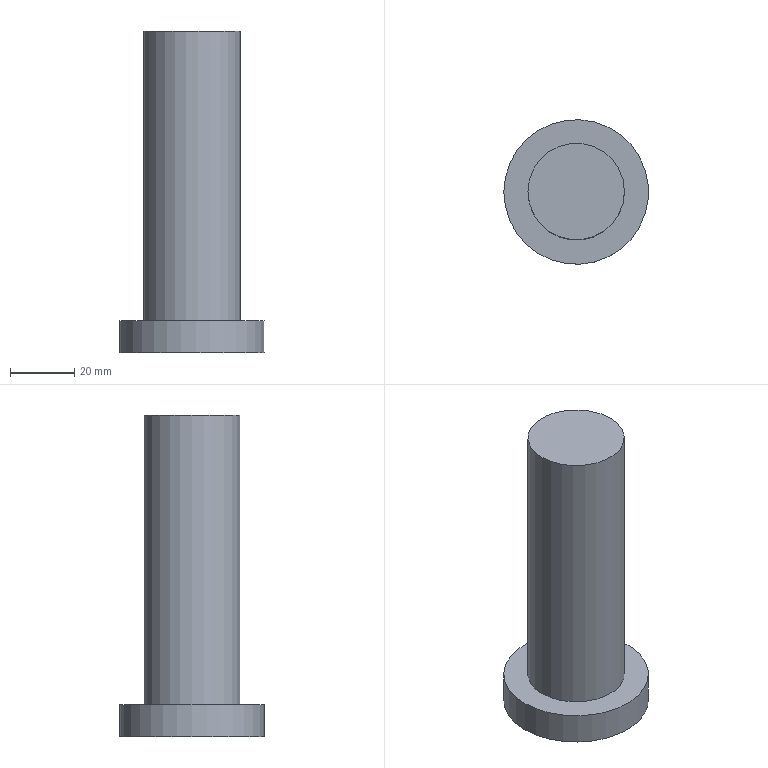Part | NX | features 侧推千斤顶缸销 2 | 1 solid | 5 faces | box 45 x 45 x 100 mm | volume 79522 mm3 | plane 3 | cylinder 2 | commonest cylinder face diameters 30 x1 45 x1
STEP:
#1=CARTESIAN_POINT('',(15.,0.,90.));
#2=VERTEX_POINT('',#1);
#3=CARTESIAN_POINT('',(0.,0.,90.));
#4=DIRECTION('',(0.,0.,1.));
#5=DIRECTION('',(1.,0.,0.));
#6=AXIS2_PLACEMENT_3D('',#3,#4,#5);
#7=CIRCLE('',#6,15.);
#8=EDGE_CURVE('',#2,#2,#7,.T.);
#9=ORIENTED_EDGE('',*,*,#8,.F.);
#10=EDGE_LOOP('',(#9));
#11=FACE_BOUND('',#10,.T.);
#12=CARTESIAN_POINT('',(-15.,0.,0.));
#13=VERTEX_POINT('',#12);
#14=CARTESIAN_POINT('',(0.,0.,0.));
#15=DIRECTION('',(0.,0.,-1.));
#16=DIRECTION('',(-1.,0.,0.));
#17=AXIS2_PLACEMENT_3D('',#14,#15,#16);
#18=CIRCLE('',#17,15.);
#19=EDGE_CURVE('',#13,#13,#18,.T.);
#20=ORIENTED_EDGE('',*,*,#19,.F.);
#21=EDGE_LOOP('',(#20));
#22=FACE_BOUND('',#21,.T.);
#23=CARTESIAN_POINT('',(0.,0.,90.));
#24=DIRECTION('',(0.,0.,-1.));
#25=DIRECTION('',(-1.,0.,0.));
#26=AXIS2_PLACEMENT_3D('',#23,#24,#25);
#27=CYLINDRICAL_SURFACE('',#26,15.);
#28=ADVANCED_FACE('',(#11,#22),#27,.T.);
#29=ORIENTED_EDGE('',*,*,#8,.T.);
#30=EDGE_LOOP('',(#29));
#31=FACE_BOUND('',#30,.T.);
#32=CARTESIAN_POINT('',(0.,0.,90.));
#33=DIRECTION('',(0.,0.,1.));
#34=DIRECTION('',(1.,0.,0.));
#35=AXIS2_PLACEMENT_3D('',#32,#33,#34);
#36=PLANE('',#35);
#37=ADVANCED_FACE('',(#31),#36,.T.);
#38=CARTESIAN_POINT('',(-22.5,0.,0.));
#39=VERTEX_POINT('',#38);
#40=CARTESIAN_POINT('',(0.,0.,0.));
#41=DIRECTION('',(0.,0.,-1.));
#42=DIRECTION('',(-1.,0.,0.));
#43=AXIS2_PLACEMENT_3D('',#40,#41,#42);
#44=CIRCLE('',#43,22.5);
#45=EDGE_CURVE('',#39,#39,#44,.T.);
#46=ORIENTED_EDGE('',*,*,#45,.F.);
#47=EDGE_LOOP('',(#46));
#48=FACE_BOUND('',#47,.T.);
#49=ORIENTED_EDGE('',*,*,#19,.T.);
#50=EDGE_LOOP('',(#49));
#51=FACE_BOUND('',#50,.T.);
#52=CARTESIAN_POINT('',(0.,0.,0.));
#53=DIRECTION('',(0.,0.,-1.));
#54=DIRECTION('',(-1.,0.,0.));
#55=AXIS2_PLACEMENT_3D('',#52,#53,#54);
#56=PLANE('',#55);
#57=ADVANCED_FACE('',(#48,#51),#56,.F.);
#58=CARTESIAN_POINT('',(-22.5,0.,-10.));
#59=VERTEX_POINT('',#58);
#60=CARTESIAN_POINT('',(0.,0.,-10.));
#61=DIRECTION('',(0.,0.,-1.));
#62=DIRECTION('',(-1.,0.,0.));
#63=AXIS2_PLACEMENT_3D('',#60,#61,#62);
#64=CIRCLE('',#63,22.5);
#65=EDGE_CURVE('',#59,#59,#64,.T.);
#66=ORIENTED_EDGE('',*,*,#65,.F.);
#67=EDGE_LOOP('',(#66));
#68=FACE_BOUND('',#67,.T.);
#69=ORIENTED_EDGE('',*,*,#45,.T.);
#70=EDGE_LOOP('',(#69));
#71=FACE_BOUND('',#70,.T.);
#72=CARTESIAN_POINT('',(0.,0.,-10.));
#73=DIRECTION('',(0.,0.,1.));
#74=DIRECTION('',(1.,0.,0.));
#75=AXIS2_PLACEMENT_3D('',#72,#73,#74);
#76=CYLINDRICAL_SURFACE('',#75,22.5);
#77=ADVANCED_FACE('',(#68,#71),#76,.T.);
#78=ORIENTED_EDGE('',*,*,#65,.T.);
#79=EDGE_LOOP('',(#78));
#80=FACE_BOUND('',#79,.T.);
#81=CARTESIAN_POINT('',(0.,0.,-10.));
#82=DIRECTION('',(0.,0.,-1.));
#83=DIRECTION('',(-1.,0.,0.));
#84=AXIS2_PLACEMENT_3D('',#81,#82,#83);
#85=PLANE('',#84);
#86=ADVANCED_FACE('',(#80),#85,.T.);
#87=CLOSED_SHELL('',(#28,#37,#57,#77,#86));
#88=MANIFOLD_SOLID_BREP('',#87);
#89=(LENGTH_UNIT()NAMED_UNIT(*)SI_UNIT(.MILLI.,.METRE.));
#90=UNCERTAINTY_MEASURE_WITH_UNIT(LENGTH_MEASURE(0.00001),#89,'','');
#91=(NAMED_UNIT(*)PLANE_ANGLE_UNIT()SI_UNIT($,.RADIAN.));
#92=(NAMED_UNIT(*)SI_UNIT($,.STERADIAN.)SOLID_ANGLE_UNIT());
#93=(GEOMETRIC_REPRESENTATION_CONTEXT(3)GLOBAL_UNCERTAINTY_ASSIGNED_CONTEXT((#90))GLOBAL_UNIT_ASSIGNED_CONTEXT((#89,#91,#92))REPRESENTATION_CONTEXT('',''));
#94=ADVANCED_BREP_SHAPE_REPRESENTATION('',(#88),#93);